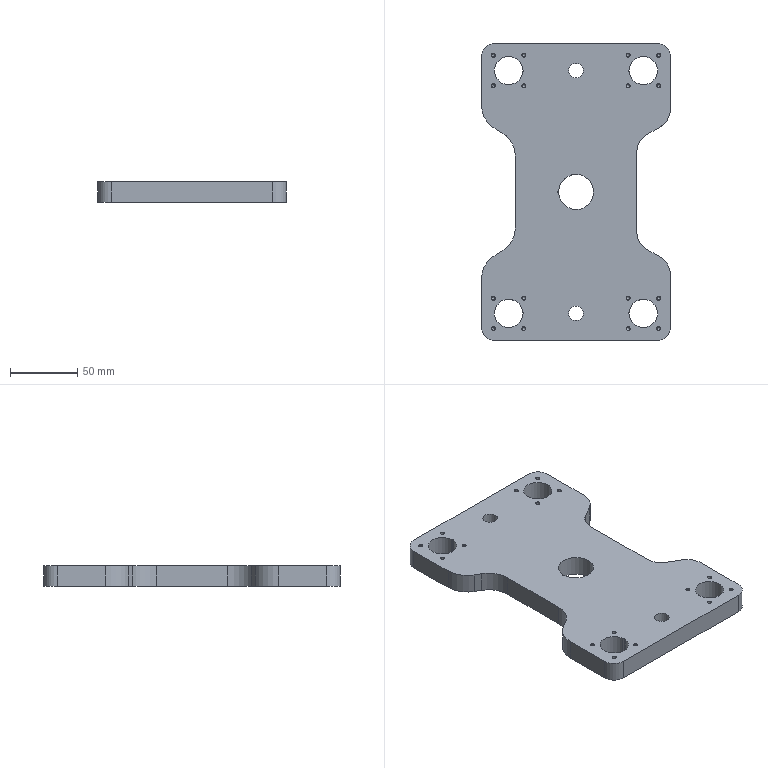Part | STEP file | YBQDJ-YL-5 | 1 solid | 96 faces | box 140 x 220 x 15 mm | volume 360572 mm3 | cylinder 50 | cone 32 | plane 14 | commonest cylinder face diameters 2.5 x16 4 x10 1 x5 20 x4 21.01 x4 30 x4